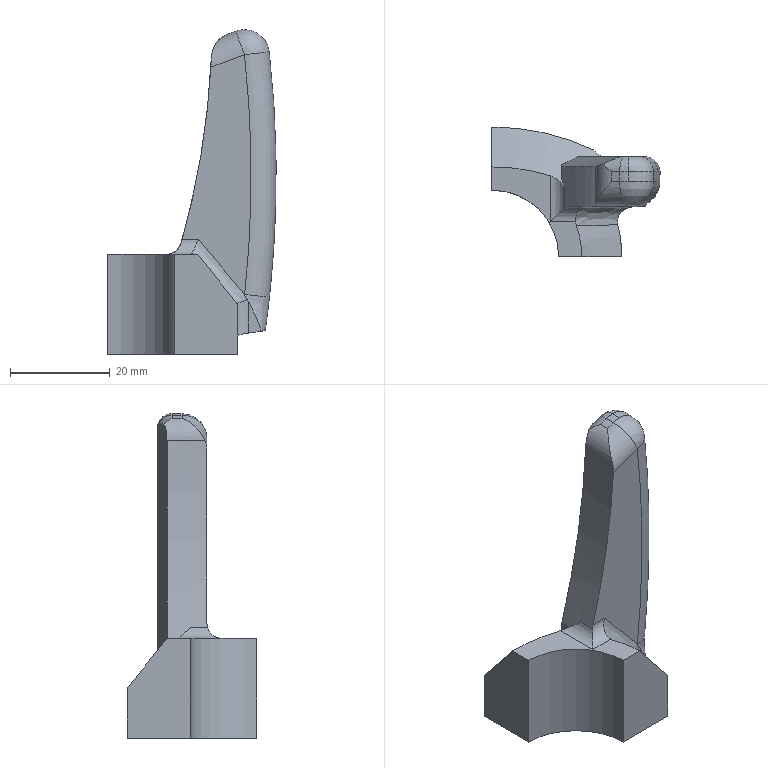Part | STEP file | Twistshift IndicatorMirror 3 speed | 1 solid | 44 faces | box 33.672 x 26 x 65.01 mm | volume 13907 mm3 | cylinder 15 | plane 13 | cone 8 | spline 3 | other 2 | torus 2 | sphere 1 | commonest cylinder face diameters 6 x6 10 x4 26.699 x1 52 x1 95 x1 326.416 x1